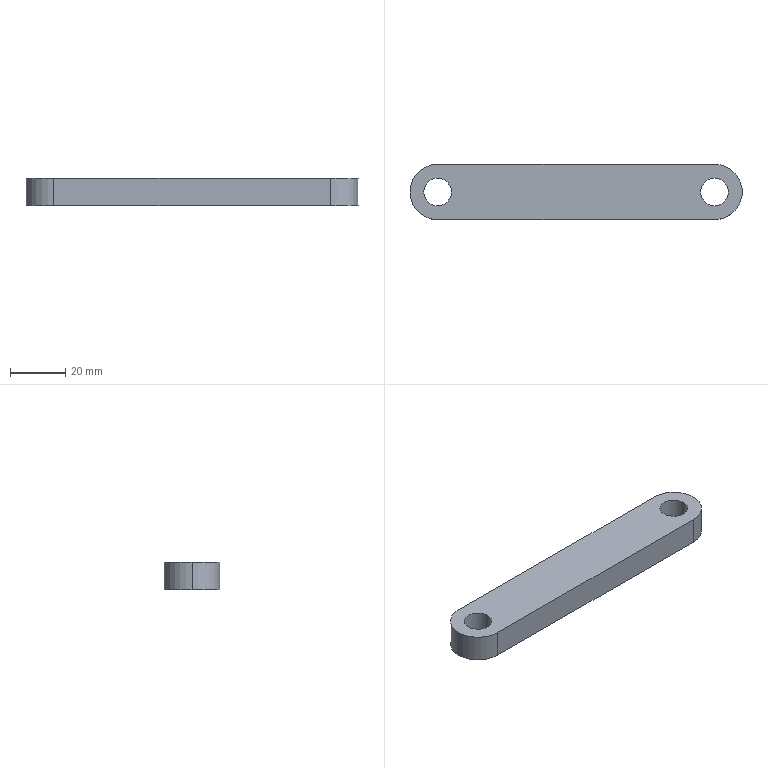Part | SolidWorks | features Extrusion 1 | 1 solid | 11 faces | box 120 x 20 x 10 mm | volume 21571 mm3 | cylinder 7 | plane 4 | commonest cylinder face diameters 10 x4 20 x3
STEP:
#1=CARTESIAN_POINT('',(-30.,0.,10.));
#2=VERTEX_POINT('',#1);
#3=CARTESIAN_POINT('',(-20.,0.,10.));
#4=VERTEX_POINT('',#3);
#5=CARTESIAN_POINT('',(-25.,0.,10.));
#6=DIRECTION('',(0.,0.,1.));
#7=DIRECTION('',(1.,0.,0.));
#8=AXIS2_PLACEMENT_3D('',#5,#6,#7);
#9=CIRCLE('',#8,5.);
#10=EDGE_CURVE('',#2,#4,#9,.T.);
#11=ORIENTED_EDGE('',*,*,#10,.T.);
#12=CARTESIAN_POINT('',(-20.,0.,0.));
#13=VERTEX_POINT('',#12);
#14=CARTESIAN_POINT('',(-20.,0.,10.));
#15=DIRECTION('',(0.,0.,-1.));
#16=VECTOR('',#15,1000.);
#17=LINE('',#14,#16);
#18=EDGE_CURVE('',#4,#13,#17,.T.);
#19=ORIENTED_EDGE('',*,*,#18,.T.);
#20=CARTESIAN_POINT('',(-30.,0.,0.));
#21=VERTEX_POINT('',#20);
#22=CARTESIAN_POINT('',(-25.,0.,0.));
#23=DIRECTION('',(0.,0.,1.));
#24=DIRECTION('',(1.,0.,0.));
#25=AXIS2_PLACEMENT_3D('',#22,#23,#24);
#26=CIRCLE('',#25,5.);
#27=EDGE_CURVE('',#21,#13,#26,.T.);
#28=ORIENTED_EDGE('',*,*,#27,.F.);
#29=CARTESIAN_POINT('',(-30.,0.,10.));
#30=DIRECTION('',(0.,0.,-1.));
#31=VECTOR('',#30,1000.);
#32=LINE('',#29,#31);
#33=EDGE_CURVE('',#2,#21,#32,.T.);
#34=ORIENTED_EDGE('',*,*,#33,.F.);
#35=EDGE_LOOP('',(#11,#19,#28,#34));
#36=FACE_OUTER_BOUND('',#35,.T.);
#37=CARTESIAN_POINT('',(-25.,0.,10.));
#38=DIRECTION('',(0.,0.,-1.));
#39=DIRECTION('',(-1.,0.,0.));
#40=AXIS2_PLACEMENT_3D('',#37,#38,#39);
#41=CYLINDRICAL_SURFACE('',#40,5.);
#42=ADVANCED_FACE('',(#36),#41,.F.);
#43=CARTESIAN_POINT('',(70.,0.,10.));
#44=VERTEX_POINT('',#43);
#45=CARTESIAN_POINT('',(80.,0.,10.));
#46=VERTEX_POINT('',#45);
#47=CARTESIAN_POINT('',(75.,0.,10.));
#48=DIRECTION('',(0.,0.,1.));
#49=DIRECTION('',(1.,0.,0.));
#50=AXIS2_PLACEMENT_3D('',#47,#48,#49);
#51=CIRCLE('',#50,5.);
#52=EDGE_CURVE('',#44,#46,#51,.T.);
#53=ORIENTED_EDGE('',*,*,#52,.T.);
#54=CARTESIAN_POINT('',(80.,0.,0.));
#55=VERTEX_POINT('',#54);
#56=CARTESIAN_POINT('',(80.,0.,10.));
#57=DIRECTION('',(0.,0.,-1.));
#58=VECTOR('',#57,1000.);
#59=LINE('',#56,#58);
#60=EDGE_CURVE('',#46,#55,#59,.T.);
#61=ORIENTED_EDGE('',*,*,#60,.T.);
#62=CARTESIAN_POINT('',(70.,0.,0.));
#63=VERTEX_POINT('',#62);
#64=CARTESIAN_POINT('',(75.,0.,0.));
#65=DIRECTION('',(0.,0.,1.));
#66=DIRECTION('',(1.,0.,0.));
#67=AXIS2_PLACEMENT_3D('',#64,#65,#66);
#68=CIRCLE('',#67,5.);
#69=EDGE_CURVE('',#63,#55,#68,.T.);
#70=ORIENTED_EDGE('',*,*,#69,.F.);
#71=CARTESIAN_POINT('',(70.,0.,10.));
#72=DIRECTION('',(0.,0.,-1.));
#73=VECTOR('',#72,1000.);
#74=LINE('',#71,#73);
#75=EDGE_CURVE('',#44,#63,#74,.T.);
#76=ORIENTED_EDGE('',*,*,#75,.F.);
#77=EDGE_LOOP('',(#53,#61,#70,#76));
#78=FACE_OUTER_BOUND('',#77,.T.);
#79=CARTESIAN_POINT('',(75.,0.,10.));
#80=DIRECTION('',(0.,0.,-1.));
#81=DIRECTION('',(-1.,0.,0.));
#82=AXIS2_PLACEMENT_3D('',#79,#80,#81);
#83=CYLINDRICAL_SURFACE('',#82,5.);
#84=ADVANCED_FACE('',(#78),#83,.F.);
#85=CARTESIAN_POINT('',(-35.,0.,10.));
#86=VERTEX_POINT('',#85);
#87=CARTESIAN_POINT('',(-25.,-10.,10.));
#88=VERTEX_POINT('',#87);
#89=CARTESIAN_POINT('',(-25.,0.,10.));
#90=DIRECTION('',(0.,0.,1.));
#91=DIRECTION('',(1.,0.,0.));
#92=AXIS2_PLACEMENT_3D('',#89,#90,#91);
#93=CIRCLE('',#92,10.);
#94=EDGE_CURVE('',#86,#88,#93,.T.);
#95=ORIENTED_EDGE('',*,*,#94,.F.);
#96=CARTESIAN_POINT('',(-35.,0.,0.));
#97=VERTEX_POINT('',#96);
#98=CARTESIAN_POINT('',(-35.,0.,10.));
#99=DIRECTION('',(0.,0.,-1.));
#100=VECTOR('',#99,1000.);
#101=LINE('',#98,#100);
#102=EDGE_CURVE('',#86,#97,#101,.T.);
#103=ORIENTED_EDGE('',*,*,#102,.T.);
#104=CARTESIAN_POINT('',(-25.,-10.,0.));
#105=VERTEX_POINT('',#104);
#106=CARTESIAN_POINT('',(-25.,0.,0.));
#107=DIRECTION('',(0.,0.,1.));
#108=DIRECTION('',(1.,0.,0.));
#109=AXIS2_PLACEMENT_3D('',#106,#107,#108);
#110=CIRCLE('',#109,10.);
#111=EDGE_CURVE('',#97,#105,#110,.T.);
#112=ORIENTED_EDGE('',*,*,#111,.T.);
#113=CARTESIAN_POINT('',(-25.,-10.,10.));
#114=DIRECTION('',(0.,0.,-1.));
#115=VECTOR('',#114,1000.);
#116=LINE('',#113,#115);
#117=EDGE_CURVE('',#88,#105,#116,.T.);
#118=ORIENTED_EDGE('',*,*,#117,.F.);
#119=EDGE_LOOP('',(#95,#103,#112,#118));
#120=FACE_OUTER_BOUND('',#119,.T.);
#121=CARTESIAN_POINT('',(-25.,0.,10.));
#122=DIRECTION('',(0.,0.,-1.));
#123=DIRECTION('',(-1.,0.,0.));
#124=AXIS2_PLACEMENT_3D('',#121,#122,#123);
#125=CYLINDRICAL_SURFACE('',#124,10.);
#126=ADVANCED_FACE('',(#120),#125,.T.);
#127=ORIENTED_EDGE('',*,*,#52,.F.);
#128=CARTESIAN_POINT('',(75.,0.,10.));
#129=DIRECTION('',(0.,0.,1.));
#130=DIRECTION('',(1.,0.,0.));
#131=AXIS2_PLACEMENT_3D('',#128,#129,#130);
#132=CIRCLE('',#131,5.);
#133=EDGE_CURVE('',#46,#44,#132,.T.);
#134=ORIENTED_EDGE('',*,*,#133,.F.);
#135=EDGE_LOOP('',(#127,#134));
#136=FACE_BOUND('',#135,.T.);
#137=CARTESIAN_POINT('',(75.,-10.,10.));
#138=VERTEX_POINT('',#137);
#139=CARTESIAN_POINT('',(75.,10.,10.));
#140=VERTEX_POINT('',#139);
#141=CARTESIAN_POINT('',(75.,0.,10.));
#142=DIRECTION('',(0.,0.,1.));
#143=DIRECTION('',(1.,0.,0.));
#144=AXIS2_PLACEMENT_3D('',#141,#142,#143);
#145=CIRCLE('',#144,10.);
#146=EDGE_CURVE('',#138,#140,#145,.T.);
#147=ORIENTED_EDGE('',*,*,#146,.T.);
#148=CARTESIAN_POINT('',(-25.,10.,10.));
#149=VERTEX_POINT('',#148);
#150=CARTESIAN_POINT('',(-25.,10.,10.));
#151=DIRECTION('',(-1.,0.,0.));
#152=VECTOR('',#151,1000.);
#153=LINE('',#150,#152);
#154=EDGE_CURVE('',#140,#149,#153,.T.);
#155=ORIENTED_EDGE('',*,*,#154,.T.);
#156=CARTESIAN_POINT('',(-25.,0.,10.));
#157=DIRECTION('',(0.,0.,1.));
#158=DIRECTION('',(1.,0.,0.));
#159=AXIS2_PLACEMENT_3D('',#156,#157,#158);
#160=CIRCLE('',#159,10.);
#161=EDGE_CURVE('',#149,#86,#160,.T.);
#162=ORIENTED_EDGE('',*,*,#161,.T.);
#163=ORIENTED_EDGE('',*,*,#94,.T.);
#164=CARTESIAN_POINT('',(-25.,-10.,10.));
#165=DIRECTION('',(1.,0.,0.));
#166=VECTOR('',#165,1000.);
#167=LINE('',#164,#166);
#168=EDGE_CURVE('',#88,#138,#167,.T.);
#169=ORIENTED_EDGE('',*,*,#168,.T.);
#170=EDGE_LOOP('',(#147,#155,#162,#163,#169));
#171=FACE_OUTER_BOUND('',#170,.T.);
#172=ORIENTED_EDGE('',*,*,#10,.F.);
#173=CARTESIAN_POINT('',(-25.,0.,10.));
#174=DIRECTION('',(0.,0.,1.));
#175=DIRECTION('',(1.,0.,0.));
#176=AXIS2_PLACEMENT_3D('',#173,#174,#175);
#177=CIRCLE('',#176,5.);
#178=EDGE_CURVE('',#4,#2,#177,.T.);
#179=ORIENTED_EDGE('',*,*,#178,.F.);
#180=EDGE_LOOP('',(#172,#179));
#181=FACE_BOUND('',#180,.T.);
#182=CARTESIAN_POINT('',(75.,0.,10.));
#183=DIRECTION('',(0.,0.,1.));
#184=DIRECTION('',(1.,0.,0.));
#185=AXIS2_PLACEMENT_3D('',#182,#183,#184);
#186=PLANE('',#185);
#187=ADVANCED_FACE('',(#136,#171,#181),#186,.T.);
#188=ORIENTED_EDGE('',*,*,#69,.T.);
#189=CARTESIAN_POINT('',(75.,0.,0.));
#190=DIRECTION('',(0.,0.,1.));
#191=DIRECTION('',(1.,0.,0.));
#192=AXIS2_PLACEMENT_3D('',#189,#190,#191);
#193=CIRCLE('',#192,5.);
#194=EDGE_CURVE('',#55,#63,#193,.T.);
#195=ORIENTED_EDGE('',*,*,#194,.T.);
#196=EDGE_LOOP('',(#188,#195));
#197=FACE_BOUND('',#196,.T.);
#198=CARTESIAN_POINT('',(75.,-10.,0.));
#199=VERTEX_POINT('',#198);
#200=CARTESIAN_POINT('',(75.,10.,0.));
#201=VERTEX_POINT('',#200);
#202=CARTESIAN_POINT('',(75.,0.,0.));
#203=DIRECTION('',(0.,0.,1.));
#204=DIRECTION('',(1.,0.,0.));
#205=AXIS2_PLACEMENT_3D('',#202,#203,#204);
#206=CIRCLE('',#205,10.);
#207=EDGE_CURVE('',#199,#201,#206,.T.);
#208=ORIENTED_EDGE('',*,*,#207,.F.);
#209=CARTESIAN_POINT('',(-25.,-10.,0.));
#210=DIRECTION('',(1.,0.,0.));
#211=VECTOR('',#210,1000.);
#212=LINE('',#209,#211);
#213=EDGE_CURVE('',#105,#199,#212,.T.);
#214=ORIENTED_EDGE('',*,*,#213,.F.);
#215=ORIENTED_EDGE('',*,*,#111,.F.);
#216=CARTESIAN_POINT('',(-25.,10.,0.));
#217=VERTEX_POINT('',#216);
#218=CARTESIAN_POINT('',(-25.,0.,0.));
#219=DIRECTION('',(0.,0.,1.));
#220=DIRECTION('',(1.,0.,0.));
#221=AXIS2_PLACEMENT_3D('',#218,#219,#220);
#222=CIRCLE('',#221,10.);
#223=EDGE_CURVE('',#217,#97,#222,.T.);
#224=ORIENTED_EDGE('',*,*,#223,.F.);
#225=CARTESIAN_POINT('',(-25.,10.,0.));
#226=DIRECTION('',(-1.,0.,0.));
#227=VECTOR('',#226,1000.);
#228=LINE('',#225,#227);
#229=EDGE_CURVE('',#201,#217,#228,.T.);
#230=ORIENTED_EDGE('',*,*,#229,.F.);
#231=EDGE_LOOP('',(#208,#214,#215,#224,#230));
#232=FACE_OUTER_BOUND('',#231,.T.);
#233=ORIENTED_EDGE('',*,*,#27,.T.);
#234=CARTESIAN_POINT('',(-25.,0.,0.));
#235=DIRECTION('',(0.,0.,1.));
#236=DIRECTION('',(1.,0.,0.));
#237=AXIS2_PLACEMENT_3D('',#234,#235,#236);
#238=CIRCLE('',#237,5.);
#239=EDGE_CURVE('',#13,#21,#238,.T.);
#240=ORIENTED_EDGE('',*,*,#239,.T.);
#241=EDGE_LOOP('',(#233,#240));
#242=FACE_BOUND('',#241,.T.);
#243=CARTESIAN_POINT('',(75.,0.,0.));
#244=DIRECTION('',(0.,0.,1.));
#245=DIRECTION('',(1.,0.,0.));
#246=AXIS2_PLACEMENT_3D('',#243,#244,#245);
#247=PLANE('',#246);
#248=ADVANCED_FACE('',(#197,#232,#242),#247,.F.);
#249=ORIENTED_EDGE('',*,*,#207,.T.);
#250=CARTESIAN_POINT('',(75.,10.,10.));
#251=DIRECTION('',(0.,0.,-1.));
#252=VECTOR('',#251,1000.);
#253=LINE('',#250,#252);
#254=EDGE_CURVE('',#140,#201,#253,.T.);
#255=ORIENTED_EDGE('',*,*,#254,.F.);
#256=ORIENTED_EDGE('',*,*,#146,.F.);
#257=CARTESIAN_POINT('',(75.,-10.,10.));
#258=DIRECTION('',(0.,0.,-1.));
#259=VECTOR('',#258,1000.);
#260=LINE('',#257,#259);
#261=EDGE_CURVE('',#138,#199,#260,.T.);
#262=ORIENTED_EDGE('',*,*,#261,.T.);
#263=EDGE_LOOP('',(#249,#255,#256,#262));
#264=FACE_OUTER_BOUND('',#263,.T.);
#265=CARTESIAN_POINT('',(75.,0.,10.));
#266=DIRECTION('',(0.,0.,-1.));
#267=DIRECTION('',(-1.,0.,0.));
#268=AXIS2_PLACEMENT_3D('',#265,#266,#267);
#269=CYLINDRICAL_SURFACE('',#268,10.);
#270=ADVANCED_FACE('',(#264),#269,.T.);
#271=ORIENTED_EDGE('',*,*,#229,.T.);
#272=CARTESIAN_POINT('',(-25.,10.,10.));
#273=DIRECTION('',(0.,0.,-1.));
#274=VECTOR('',#273,1000.);
#275=LINE('',#272,#274);
#276=EDGE_CURVE('',#149,#217,#275,.T.);
#277=ORIENTED_EDGE('',*,*,#276,.F.);
#278=ORIENTED_EDGE('',*,*,#154,.F.);
#279=ORIENTED_EDGE('',*,*,#254,.T.);
#280=EDGE_LOOP('',(#271,#277,#278,#279));
#281=FACE_OUTER_BOUND('',#280,.T.);
#282=CARTESIAN_POINT('',(-25.,10.,10.));
#283=DIRECTION('',(0.,-1.,0.));
#284=DIRECTION('',(0.,0.,-1.));
#285=AXIS2_PLACEMENT_3D('',#282,#283,#284);
#286=PLANE('',#285);
#287=ADVANCED_FACE('',(#281),#286,.F.);
#288=ORIENTED_EDGE('',*,*,#102,.F.);
#289=ORIENTED_EDGE('',*,*,#161,.F.);
#290=ORIENTED_EDGE('',*,*,#276,.T.);
#291=ORIENTED_EDGE('',*,*,#223,.T.);
#292=EDGE_LOOP('',(#288,#289,#290,#291));
#293=FACE_OUTER_BOUND('',#292,.T.);
#294=CARTESIAN_POINT('',(-25.,0.,10.));
#295=DIRECTION('',(0.,0.,-1.));
#296=DIRECTION('',(-1.,0.,0.));
#297=AXIS2_PLACEMENT_3D('',#294,#295,#296);
#298=CYLINDRICAL_SURFACE('',#297,10.);
#299=ADVANCED_FACE('',(#293),#298,.T.);
#300=ORIENTED_EDGE('',*,*,#213,.T.);
#301=ORIENTED_EDGE('',*,*,#261,.F.);
#302=ORIENTED_EDGE('',*,*,#168,.F.);
#303=ORIENTED_EDGE('',*,*,#117,.T.);
#304=EDGE_LOOP('',(#300,#301,#302,#303));
#305=FACE_OUTER_BOUND('',#304,.T.);
#306=CARTESIAN_POINT('',(-25.,-10.,10.));
#307=DIRECTION('',(0.,1.,0.));
#308=DIRECTION('',(0.,0.,1.));
#309=AXIS2_PLACEMENT_3D('',#306,#307,#308);
#310=PLANE('',#309);
#311=ADVANCED_FACE('',(#305),#310,.F.);
#312=ORIENTED_EDGE('',*,*,#60,.F.);
#313=ORIENTED_EDGE('',*,*,#133,.T.);
#314=ORIENTED_EDGE('',*,*,#75,.T.);
#315=ORIENTED_EDGE('',*,*,#194,.F.);
#316=EDGE_LOOP('',(#312,#313,#314,#315));
#317=FACE_OUTER_BOUND('',#316,.T.);
#318=CARTESIAN_POINT('',(75.,0.,10.));
#319=DIRECTION('',(0.,0.,-1.));
#320=DIRECTION('',(-1.,0.,0.));
#321=AXIS2_PLACEMENT_3D('',#318,#319,#320);
#322=CYLINDRICAL_SURFACE('',#321,5.);
#323=ADVANCED_FACE('',(#317),#322,.F.);
#324=ORIENTED_EDGE('',*,*,#18,.F.);
#325=ORIENTED_EDGE('',*,*,#178,.T.);
#326=ORIENTED_EDGE('',*,*,#33,.T.);
#327=ORIENTED_EDGE('',*,*,#239,.F.);
#328=EDGE_LOOP('',(#324,#325,#326,#327));
#329=FACE_OUTER_BOUND('',#328,.T.);
#330=CARTESIAN_POINT('',(-25.,0.,10.));
#331=DIRECTION('',(0.,0.,-1.));
#332=DIRECTION('',(-1.,0.,0.));
#333=AXIS2_PLACEMENT_3D('',#330,#331,#332);
#334=CYLINDRICAL_SURFACE('',#333,5.);
#335=ADVANCED_FACE('',(#329),#334,.F.);
#336=CLOSED_SHELL('',(#42,#84,#126,#187,#248,#270,#287,#299,#311,#323,#335));
#337=MANIFOLD_SOLID_BREP('',#336);
#338=CARTESIAN_POINT('',(0.,0.,0.));
#339=DIRECTION('',(0.,0.,1.));
#340=DIRECTION('',(1.,0.,0.));
#341=AXIS2_PLACEMENT_3D('',#338,#339,#340);
#342=(LENGTH_UNIT()NAMED_UNIT(*)SI_UNIT(.MILLI.,.METRE.));
#343=UNCERTAINTY_MEASURE_WITH_UNIT(LENGTH_MEASURE(0.00001),#342,'','');
#344=(NAMED_UNIT(*)PLANE_ANGLE_UNIT()SI_UNIT($,.RADIAN.));
#345=(NAMED_UNIT(*)SI_UNIT($,.STERADIAN.)SOLID_ANGLE_UNIT());
#346=(GEOMETRIC_REPRESENTATION_CONTEXT(3)GLOBAL_UNCERTAINTY_ASSIGNED_CONTEXT((#343))GLOBAL_UNIT_ASSIGNED_CONTEXT((#342,#344,#345))REPRESENTATION_CONTEXT('',''));
#347=ADVANCED_BREP_SHAPE_REPRESENTATION('',(#337,#341),#346);